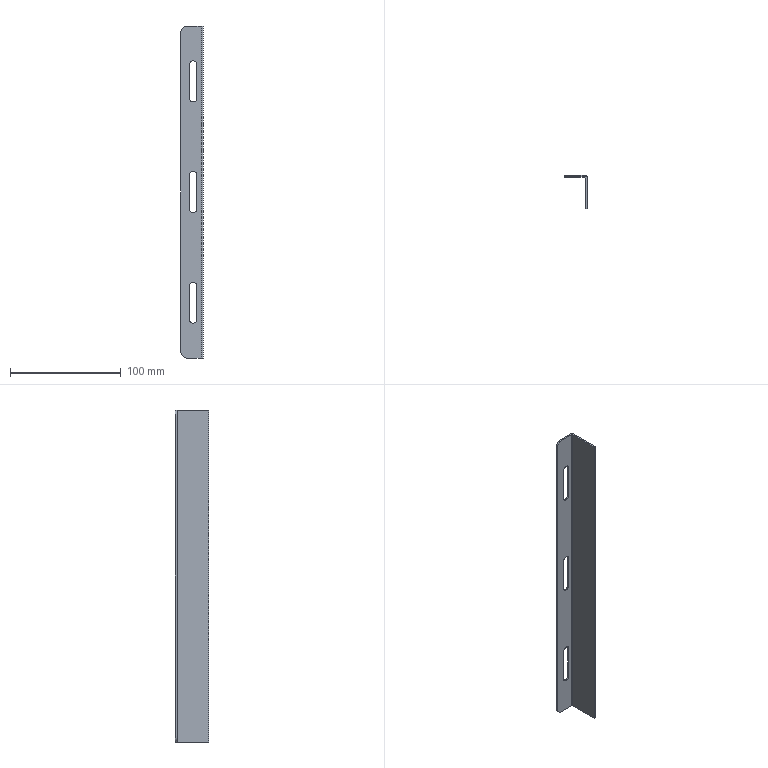Part | SolidWorks | features Cut 1, Fillet 1, FlatPattern 1, SMBaseFlange 1, SheetMetal 1 | 1 solid | 31 faces | box 20 x 30 x 300 mm | volume 20507 mm3 | plane 18 | cylinder 13 | commonest cylinder face diameters 7 x9 10 x2 0.4 x1 3.4 x1
STEP:
#1=CARTESIAN_POINT('',(-9.,-1.5,118.5));
#2=VERTEX_POINT('',#1);
#3=CARTESIAN_POINT('',(-5.5,-1.5,115.));
#4=VERTEX_POINT('',#3);
#5=CARTESIAN_POINT('',(-9.,-1.5,115.));
#6=DIRECTION('',(0.,1.,0.));
#7=DIRECTION('',(-1.,0.,0.));
#8=AXIS2_PLACEMENT_3D('',#5,#6,#7);
#9=CIRCLE('',#8,3.5);
#10=EDGE_CURVE('',#2,#4,#9,.T.);
#11=ORIENTED_EDGE('',*,*,#10,.F.);
#12=CARTESIAN_POINT('',(-9.,0.,118.5));
#13=VERTEX_POINT('',#12);
#14=CARTESIAN_POINT('',(-9.,-10.,118.5));
#15=DIRECTION('',(0.,1.,0.));
#16=VECTOR('',#15,1000.);
#17=LINE('',#14,#16);
#18=EDGE_CURVE('',#2,#13,#17,.T.);
#19=ORIENTED_EDGE('',*,*,#18,.T.);
#20=CARTESIAN_POINT('',(-5.5,0.,115.));
#21=VERTEX_POINT('',#20);
#22=CARTESIAN_POINT('',(-9.,0.,115.));
#23=DIRECTION('',(0.,1.,0.));
#24=DIRECTION('',(0.,0.,-1.));
#25=AXIS2_PLACEMENT_3D('',#22,#23,#24);
#26=CIRCLE('',#25,3.5);
#27=EDGE_CURVE('',#13,#21,#26,.T.);
#28=ORIENTED_EDGE('',*,*,#27,.T.);
#29=CARTESIAN_POINT('',(-5.5,-10.,115.));
#30=DIRECTION('',(0.,1.,0.));
#31=VECTOR('',#30,1000.);
#32=LINE('',#29,#31);
#33=EDGE_CURVE('',#4,#21,#32,.T.);
#34=ORIENTED_EDGE('',*,*,#33,.F.);
#35=EDGE_LOOP('',(#11,#19,#28,#34));
#36=FACE_OUTER_BOUND('',#35,.T.);
#37=CARTESIAN_POINT('',(-9.,-10.,115.));
#38=DIRECTION('',(0.,1.,0.));
#39=DIRECTION('',(0.,0.,1.));
#40=AXIS2_PLACEMENT_3D('',#37,#38,#39);
#41=CYLINDRICAL_SURFACE('',#40,3.5);
#42=ADVANCED_FACE('',(#36),#41,.F.);
#43=CARTESIAN_POINT('',(-9.,-1.5,-81.5));
#44=VERTEX_POINT('',#43);
#45=CARTESIAN_POINT('',(-5.5,-1.5,-85.));
#46=VERTEX_POINT('',#45);
#47=CARTESIAN_POINT('',(-9.,-1.5,-85.));
#48=DIRECTION('',(0.,1.,0.));
#49=DIRECTION('',(-1.,0.,0.));
#50=AXIS2_PLACEMENT_3D('',#47,#48,#49);
#51=CIRCLE('',#50,3.5);
#52=EDGE_CURVE('',#44,#46,#51,.T.);
#53=ORIENTED_EDGE('',*,*,#52,.F.);
#54=CARTESIAN_POINT('',(-9.,0.,-81.5));
#55=VERTEX_POINT('',#54);
#56=CARTESIAN_POINT('',(-9.,-10.,-81.5));
#57=DIRECTION('',(0.,1.,0.));
#58=VECTOR('',#57,1000.);
#59=LINE('',#56,#58);
#60=EDGE_CURVE('',#44,#55,#59,.T.);
#61=ORIENTED_EDGE('',*,*,#60,.T.);
#62=CARTESIAN_POINT('',(-5.5,0.,-85.));
#63=VERTEX_POINT('',#62);
#64=CARTESIAN_POINT('',(-9.,0.,-85.));
#65=DIRECTION('',(0.,1.,0.));
#66=DIRECTION('',(0.,0.,1.));
#67=AXIS2_PLACEMENT_3D('',#64,#65,#66);
#68=CIRCLE('',#67,3.5);
#69=EDGE_CURVE('',#55,#63,#68,.T.);
#70=ORIENTED_EDGE('',*,*,#69,.T.);
#71=CARTESIAN_POINT('',(-5.5,-10.,-85.));
#72=DIRECTION('',(0.,1.,0.));
#73=VECTOR('',#72,1000.);
#74=LINE('',#71,#73);
#75=EDGE_CURVE('',#46,#63,#74,.T.);
#76=ORIENTED_EDGE('',*,*,#75,.F.);
#77=EDGE_LOOP('',(#53,#61,#70,#76));
#78=FACE_OUTER_BOUND('',#77,.T.);
#79=CARTESIAN_POINT('',(-9.,-10.,-85.));
#80=DIRECTION('',(0.,1.,0.));
#81=DIRECTION('',(0.,0.,1.));
#82=AXIS2_PLACEMENT_3D('',#79,#80,#81);
#83=CYLINDRICAL_SURFACE('',#82,3.5);
#84=ADVANCED_FACE('',(#78),#83,.F.);
#85=CARTESIAN_POINT('',(-9.,-1.5,18.5));
#86=VERTEX_POINT('',#85);
#87=CARTESIAN_POINT('',(-5.5,-1.5,15.));
#88=VERTEX_POINT('',#87);
#89=CARTESIAN_POINT('',(-9.,-1.5,15.));
#90=DIRECTION('',(0.,1.,0.));
#91=DIRECTION('',(-1.,0.,0.));
#92=AXIS2_PLACEMENT_3D('',#89,#90,#91);
#93=CIRCLE('',#92,3.5);
#94=EDGE_CURVE('',#86,#88,#93,.T.);
#95=ORIENTED_EDGE('',*,*,#94,.F.);
#96=CARTESIAN_POINT('',(-9.,0.,18.5));
#97=VERTEX_POINT('',#96);
#98=CARTESIAN_POINT('',(-9.,-10.,18.5));
#99=DIRECTION('',(0.,1.,0.));
#100=VECTOR('',#99,1000.);
#101=LINE('',#98,#100);
#102=EDGE_CURVE('',#86,#97,#101,.T.);
#103=ORIENTED_EDGE('',*,*,#102,.T.);
#104=CARTESIAN_POINT('',(-5.5,0.,15.));
#105=VERTEX_POINT('',#104);
#106=CARTESIAN_POINT('',(-9.,0.,15.));
#107=DIRECTION('',(0.,1.,0.));
#108=DIRECTION('',(0.,0.,1.));
#109=AXIS2_PLACEMENT_3D('',#106,#107,#108);
#110=CIRCLE('',#109,3.5);
#111=EDGE_CURVE('',#97,#105,#110,.T.);
#112=ORIENTED_EDGE('',*,*,#111,.T.);
#113=CARTESIAN_POINT('',(-5.5,-10.,15.));
#114=DIRECTION('',(0.,1.,0.));
#115=VECTOR('',#114,1000.);
#116=LINE('',#113,#115);
#117=EDGE_CURVE('',#88,#105,#116,.T.);
#118=ORIENTED_EDGE('',*,*,#117,.F.);
#119=EDGE_LOOP('',(#95,#103,#112,#118));
#120=FACE_OUTER_BOUND('',#119,.T.);
#121=CARTESIAN_POINT('',(-9.,-10.,15.));
#122=DIRECTION('',(0.,1.,0.));
#123=DIRECTION('',(0.,0.,1.));
#124=AXIS2_PLACEMENT_3D('',#121,#122,#123);
#125=CYLINDRICAL_SURFACE('',#124,3.5);
#126=ADVANCED_FACE('',(#120),#125,.F.);
#127=CARTESIAN_POINT('',(0.,-1.7,150.));
#128=VERTEX_POINT('',#127);
#129=CARTESIAN_POINT('',(-1.5,-1.7,150.));
#130=VERTEX_POINT('',#129);
#131=CARTESIAN_POINT('',(0.,-1.7,150.));
#132=DIRECTION('',(-1.,0.,0.));
#133=VECTOR('',#132,1000.);
#134=LINE('',#131,#133);
#135=EDGE_CURVE('',#128,#130,#134,.T.);
#136=ORIENTED_EDGE('',*,*,#135,.F.);
#137=CARTESIAN_POINT('',(-1.7,0.,150.));
#138=VERTEX_POINT('',#137);
#139=CARTESIAN_POINT('',(-1.7,-1.7,150.));
#140=DIRECTION('',(0.,0.,-1.));
#141=DIRECTION('',(1.,0.,0.));
#142=AXIS2_PLACEMENT_3D('',#139,#140,#141);
#143=CIRCLE('',#142,1.7);
#144=EDGE_CURVE('',#138,#128,#143,.T.);
#145=ORIENTED_EDGE('',*,*,#144,.F.);
#146=CARTESIAN_POINT('',(-1.7,-1.5,150.));
#147=VERTEX_POINT('',#146);
#148=CARTESIAN_POINT('',(-1.7,-1.5,150.));
#149=DIRECTION('',(0.,1.,0.));
#150=VECTOR('',#149,1000.);
#151=LINE('',#148,#150);
#152=EDGE_CURVE('',#147,#138,#151,.T.);
#153=ORIENTED_EDGE('',*,*,#152,.F.);
#154=CARTESIAN_POINT('',(-1.7,-1.7,150.));
#155=DIRECTION('',(0.,0.,-1.));
#156=DIRECTION('',(1.,0.,0.));
#157=AXIS2_PLACEMENT_3D('',#154,#155,#156);
#158=CIRCLE('',#157,0.2);
#159=EDGE_CURVE('',#147,#130,#158,.T.);
#160=ORIENTED_EDGE('',*,*,#159,.T.);
#161=EDGE_LOOP('',(#136,#145,#153,#160));
#162=FACE_OUTER_BOUND('',#161,.T.);
#163=CARTESIAN_POINT('',(0.,-1.7,150.));
#164=DIRECTION('',(0.,0.,1.));
#165=DIRECTION('',(1.,0.,0.));
#166=AXIS2_PLACEMENT_3D('',#163,#164,#165);
#167=PLANE('',#166);
#168=ADVANCED_FACE('',(#162),#167,.T.);
#169=CARTESIAN_POINT('',(0.,-30.,150.));
#170=VERTEX_POINT('',#169);
#171=CARTESIAN_POINT('',(0.,0.,150.));
#172=DIRECTION('',(0.,-1.,0.));
#173=VECTOR('',#172,1000.);
#174=LINE('',#171,#173);
#175=EDGE_CURVE('',#128,#170,#174,.T.);
#176=ORIENTED_EDGE('',*,*,#175,.F.);
#177=ORIENTED_EDGE('',*,*,#135,.T.);
#178=CARTESIAN_POINT('',(-1.5,-30.,150.));
#179=VERTEX_POINT('',#178);
#180=CARTESIAN_POINT('',(-1.5,0.,150.));
#181=DIRECTION('',(0.,-1.,0.));
#182=VECTOR('',#181,1000.);
#183=LINE('',#180,#182);
#184=EDGE_CURVE('',#130,#179,#183,.T.);
#185=ORIENTED_EDGE('',*,*,#184,.T.);
#186=CARTESIAN_POINT('',(0.,-30.,150.));
#187=DIRECTION('',(-1.,0.,0.));
#188=VECTOR('',#187,1000.);
#189=LINE('',#186,#188);
#190=EDGE_CURVE('',#170,#179,#189,.T.);
#191=ORIENTED_EDGE('',*,*,#190,.F.);
#192=EDGE_LOOP('',(#176,#177,#185,#191));
#193=FACE_OUTER_BOUND('',#192,.T.);
#194=CARTESIAN_POINT('',(-1.7,-1.5,150.));
#195=DIRECTION('',(0.,0.,1.));
#196=DIRECTION('',(1.,0.,0.));
#197=AXIS2_PLACEMENT_3D('',#194,#195,#196);
#198=PLANE('',#197);
#199=ADVANCED_FACE('',(#193),#198,.T.);
#200=CARTESIAN_POINT('',(-1.7,0.,-150.));
#201=VERTEX_POINT('',#200);
#202=CARTESIAN_POINT('',(-1.7,-1.5,-150.));
#203=VERTEX_POINT('',#202);
#204=CARTESIAN_POINT('',(-1.7,0.,-150.));
#205=DIRECTION('',(0.,-1.,0.));
#206=VECTOR('',#205,1000.);
#207=LINE('',#204,#206);
#208=EDGE_CURVE('',#201,#203,#207,.T.);
#209=ORIENTED_EDGE('',*,*,#208,.F.);
#210=CARTESIAN_POINT('',(0.,-1.7,-150.));
#211=VERTEX_POINT('',#210);
#212=CARTESIAN_POINT('',(-1.7,-1.7,-150.));
#213=DIRECTION('',(0.,0.,-1.));
#214=DIRECTION('',(1.,0.,0.));
#215=AXIS2_PLACEMENT_3D('',#212,#213,#214);
#216=CIRCLE('',#215,1.7);
#217=EDGE_CURVE('',#201,#211,#216,.T.);
#218=ORIENTED_EDGE('',*,*,#217,.T.);
#219=CARTESIAN_POINT('',(-1.5,-1.7,-150.));
#220=VERTEX_POINT('',#219);
#221=CARTESIAN_POINT('',(-1.5,-1.7,-150.));
#222=DIRECTION('',(1.,0.,0.));
#223=VECTOR('',#222,1000.);
#224=LINE('',#221,#223);
#225=EDGE_CURVE('',#220,#211,#224,.T.);
#226=ORIENTED_EDGE('',*,*,#225,.F.);
#227=CARTESIAN_POINT('',(-1.7,-1.7,-150.));
#228=DIRECTION('',(0.,0.,-1.));
#229=DIRECTION('',(1.,0.,0.));
#230=AXIS2_PLACEMENT_3D('',#227,#228,#229);
#231=CIRCLE('',#230,0.2);
#232=EDGE_CURVE('',#203,#220,#231,.T.);
#233=ORIENTED_EDGE('',*,*,#232,.F.);
#234=EDGE_LOOP('',(#209,#218,#226,#233));
#235=FACE_OUTER_BOUND('',#234,.T.);
#236=CARTESIAN_POINT('',(-1.7,0.,-150.));
#237=DIRECTION('',(0.,0.,-1.));
#238=DIRECTION('',(-1.,0.,0.));
#239=AXIS2_PLACEMENT_3D('',#236,#237,#238);
#240=PLANE('',#239);
#241=ADVANCED_FACE('',(#235),#240,.T.);
#242=CARTESIAN_POINT('',(-15.,-1.5,-150.));
#243=VERTEX_POINT('',#242);
#244=CARTESIAN_POINT('',(0.,-1.5,-150.));
#245=DIRECTION('',(1.,0.,0.));
#246=VECTOR('',#245,1000.);
#247=LINE('',#244,#246);
#248=EDGE_CURVE('',#243,#203,#247,.T.);
#249=ORIENTED_EDGE('',*,*,#248,.F.);
#250=CARTESIAN_POINT('',(-15.,0.,-150.));
#251=VERTEX_POINT('',#250);
#252=CARTESIAN_POINT('',(-15.,-1.7,-150.));
#253=DIRECTION('',(0.,1.,0.));
#254=VECTOR('',#253,1000.);
#255=LINE('',#252,#254);
#256=EDGE_CURVE('',#243,#251,#255,.T.);
#257=ORIENTED_EDGE('',*,*,#256,.T.);
#258=CARTESIAN_POINT('',(0.,0.,-150.));
#259=DIRECTION('',(1.,0.,0.));
#260=VECTOR('',#259,1000.);
#261=LINE('',#258,#260);
#262=EDGE_CURVE('',#251,#201,#261,.T.);
#263=ORIENTED_EDGE('',*,*,#262,.T.);
#264=ORIENTED_EDGE('',*,*,#208,.T.);
#265=EDGE_LOOP('',(#249,#257,#263,#264));
#266=FACE_OUTER_BOUND('',#265,.T.);
#267=CARTESIAN_POINT('',(-1.5,-1.7,-150.));
#268=DIRECTION('',(0.,0.,-1.));
#269=DIRECTION('',(-1.,0.,0.));
#270=AXIS2_PLACEMENT_3D('',#267,#268,#269);
#271=PLANE('',#270);
#272=ADVANCED_FACE('',(#266),#271,.T.);
#273=CARTESIAN_POINT('',(-1.5,-30.,-150.));
#274=VERTEX_POINT('',#273);
#275=CARTESIAN_POINT('',(-1.5,0.,-150.));
#276=DIRECTION('',(0.,-1.,0.));
#277=VECTOR('',#276,1000.);
#278=LINE('',#275,#277);
#279=EDGE_CURVE('',#220,#274,#278,.T.);
#280=ORIENTED_EDGE('',*,*,#279,.T.);
#281=CARTESIAN_POINT('',(-1.5,-30.,150.));
#282=DIRECTION('',(0.,0.,-1.));
#283=VECTOR('',#282,1000.);
#284=LINE('',#281,#283);
#285=EDGE_CURVE('',#179,#274,#284,.T.);
#286=ORIENTED_EDGE('',*,*,#285,.F.);
#287=ORIENTED_EDGE('',*,*,#184,.F.);
#288=CARTESIAN_POINT('',(-1.5,-1.7,150.));
#289=DIRECTION('',(0.,0.,-1.));
#290=VECTOR('',#289,1000.);
#291=LINE('',#288,#290);
#292=EDGE_CURVE('',#130,#220,#291,.T.);
#293=ORIENTED_EDGE('',*,*,#292,.T.);
#294=EDGE_LOOP('',(#280,#286,#287,#293));
#295=FACE_OUTER_BOUND('',#294,.T.);
#296=CARTESIAN_POINT('',(-1.5,0.,150.));
#297=DIRECTION('',(1.,0.,0.));
#298=DIRECTION('',(0.,1.,0.));
#299=AXIS2_PLACEMENT_3D('',#296,#297,#298);
#300=PLANE('',#299);
#301=ADVANCED_FACE('',(#295),#300,.F.);
#302=CARTESIAN_POINT('',(0.,-30.,-150.));
#303=VERTEX_POINT('',#302);
#304=CARTESIAN_POINT('',(0.,-30.,-150.));
#305=DIRECTION('',(-1.,0.,0.));
#306=VECTOR('',#305,1000.);
#307=LINE('',#304,#306);
#308=EDGE_CURVE('',#303,#274,#307,.T.);
#309=ORIENTED_EDGE('',*,*,#308,.F.);
#310=CARTESIAN_POINT('',(0.,-30.,150.));
#311=DIRECTION('',(0.,0.,-1.));
#312=VECTOR('',#311,1000.);
#313=LINE('',#310,#312);
#314=EDGE_CURVE('',#170,#303,#313,.T.);
#315=ORIENTED_EDGE('',*,*,#314,.F.);
#316=ORIENTED_EDGE('',*,*,#190,.T.);
#317=ORIENTED_EDGE('',*,*,#285,.T.);
#318=EDGE_LOOP('',(#309,#315,#316,#317));
#319=FACE_OUTER_BOUND('',#318,.T.);
#320=CARTESIAN_POINT('',(0.,-30.,150.));
#321=DIRECTION('',(0.,-1.,0.));
#322=DIRECTION('',(0.,0.,-1.));
#323=AXIS2_PLACEMENT_3D('',#320,#321,#322);
#324=PLANE('',#323);
#325=ADVANCED_FACE('',(#319),#324,.T.);
#326=CARTESIAN_POINT('',(0.,0.,-150.));
#327=DIRECTION('',(0.,-1.,0.));
#328=VECTOR('',#327,1000.);
#329=LINE('',#326,#328);
#330=EDGE_CURVE('',#211,#303,#329,.T.);
#331=ORIENTED_EDGE('',*,*,#330,.F.);
#332=CARTESIAN_POINT('',(0.,-1.7,150.));
#333=DIRECTION('',(0.,0.,-1.));
#334=VECTOR('',#333,1000.);
#335=LINE('',#332,#334);
#336=EDGE_CURVE('',#128,#211,#335,.T.);
#337=ORIENTED_EDGE('',*,*,#336,.F.);
#338=ORIENTED_EDGE('',*,*,#175,.T.);
#339=ORIENTED_EDGE('',*,*,#314,.T.);
#340=EDGE_LOOP('',(#331,#337,#338,#339));
#341=FACE_OUTER_BOUND('',#340,.T.);
#342=CARTESIAN_POINT('',(0.,0.,150.));
#343=DIRECTION('',(1.,0.,0.));
#344=DIRECTION('',(0.,1.,0.));
#345=AXIS2_PLACEMENT_3D('',#342,#343,#344);
#346=PLANE('',#345);
#347=ADVANCED_FACE('',(#341),#346,.T.);
#348=ORIENTED_EDGE('',*,*,#217,.F.);
#349=CARTESIAN_POINT('',(-1.7,0.,150.));
#350=DIRECTION('',(0.,0.,-1.));
#351=VECTOR('',#350,1000.);
#352=LINE('',#349,#351);
#353=EDGE_CURVE('',#138,#201,#352,.T.);
#354=ORIENTED_EDGE('',*,*,#353,.F.);
#355=ORIENTED_EDGE('',*,*,#144,.T.);
#356=ORIENTED_EDGE('',*,*,#336,.T.);
#357=EDGE_LOOP('',(#348,#354,#355,#356));
#358=FACE_OUTER_BOUND('',#357,.T.);
#359=CARTESIAN_POINT('',(-1.7,-1.7,150.));
#360=DIRECTION('',(0.,0.,-1.));
#361=DIRECTION('',(-1.,0.,0.));
#362=AXIS2_PLACEMENT_3D('',#359,#360,#361);
#363=CYLINDRICAL_SURFACE('',#362,1.7);
#364=ADVANCED_FACE('',(#358),#363,.T.);
#365=CARTESIAN_POINT('',(-5.5,0.,85.));
#366=VERTEX_POINT('',#365);
#367=CARTESIAN_POINT('',(-12.5,0.,85.));
#368=VERTEX_POINT('',#367);
#369=CARTESIAN_POINT('',(-9.,0.,85.));
#370=DIRECTION('',(0.,1.,0.));
#371=DIRECTION('',(0.,0.,-1.));
#372=AXIS2_PLACEMENT_3D('',#369,#370,#371);
#373=CIRCLE('',#372,3.5);
#374=EDGE_CURVE('',#366,#368,#373,.T.);
#375=ORIENTED_EDGE('',*,*,#374,.F.);
#376=CARTESIAN_POINT('',(-5.5,0.,85.));
#377=DIRECTION('',(0.,0.,-1.));
#378=VECTOR('',#377,1000.);
#379=LINE('',#376,#378);
#380=EDGE_CURVE('',#21,#366,#379,.T.);
#381=ORIENTED_EDGE('',*,*,#380,.F.);
#382=ORIENTED_EDGE('',*,*,#27,.F.);
#383=CARTESIAN_POINT('',(-12.5,0.,115.));
#384=VERTEX_POINT('',#383);
#385=CARTESIAN_POINT('',(-9.,0.,115.));
#386=DIRECTION('',(0.,1.,0.));
#387=DIRECTION('',(0.,0.,-1.));
#388=AXIS2_PLACEMENT_3D('',#385,#386,#387);
#389=CIRCLE('',#388,3.5);
#390=EDGE_CURVE('',#384,#13,#389,.T.);
#391=ORIENTED_EDGE('',*,*,#390,.F.);
#392=CARTESIAN_POINT('',(-12.5,0.,85.));
#393=DIRECTION('',(0.,0.,1.));
#394=VECTOR('',#393,1000.);
#395=LINE('',#392,#394);
#396=EDGE_CURVE('',#368,#384,#395,.T.);
#397=ORIENTED_EDGE('',*,*,#396,.F.);
#398=EDGE_LOOP('',(#375,#381,#382,#391,#397));
#399=FACE_BOUND('',#398,.T.);
#400=CARTESIAN_POINT('',(-12.5,0.,-85.));
#401=VERTEX_POINT('',#400);
#402=CARTESIAN_POINT('',(-9.,0.,-85.));
#403=DIRECTION('',(0.,1.,0.));
#404=DIRECTION('',(0.,0.,1.));
#405=AXIS2_PLACEMENT_3D('',#402,#403,#404);
#406=CIRCLE('',#405,3.5);
#407=EDGE_CURVE('',#401,#55,#406,.T.);
#408=ORIENTED_EDGE('',*,*,#407,.F.);
#409=CARTESIAN_POINT('',(-12.5,0.,-115.));
#410=VERTEX_POINT('',#409);
#411=CARTESIAN_POINT('',(-12.5,0.,-85.));
#412=DIRECTION('',(0.,0.,1.));
#413=VECTOR('',#412,1000.);
#414=LINE('',#411,#413);
#415=EDGE_CURVE('',#410,#401,#414,.T.);
#416=ORIENTED_EDGE('',*,*,#415,.F.);
#417=CARTESIAN_POINT('',(-5.5,0.,-115.));
#418=VERTEX_POINT('',#417);
#419=CARTESIAN_POINT('',(-9.,0.,-115.));
#420=DIRECTION('',(0.,1.,0.));
#421=DIRECTION('',(0.,0.,1.));
#422=AXIS2_PLACEMENT_3D('',#419,#420,#421);
#423=CIRCLE('',#422,3.5);
#424=EDGE_CURVE('',#418,#410,#423,.T.);
#425=ORIENTED_EDGE('',*,*,#424,.F.);
#426=CARTESIAN_POINT('',(-5.5,0.,-85.));
#427=DIRECTION('',(0.,0.,-1.));
#428=VECTOR('',#427,1000.);
#429=LINE('',#426,#428);
#430=EDGE_CURVE('',#63,#418,#429,.T.);
#431=ORIENTED_EDGE('',*,*,#430,.F.);
#432=ORIENTED_EDGE('',*,*,#69,.F.);
#433=EDGE_LOOP('',(#408,#416,#425,#431,#432));
#434=FACE_BOUND('',#433,.T.);
#435=CARTESIAN_POINT('',(-12.5,0.,15.));
#436=VERTEX_POINT('',#435);
#437=CARTESIAN_POINT('',(-9.,0.,15.));
#438=DIRECTION('',(0.,1.,0.));
#439=DIRECTION('',(0.,0.,1.));
#440=AXIS2_PLACEMENT_3D('',#437,#438,#439);
#441=CIRCLE('',#440,3.5);
#442=EDGE_CURVE('',#436,#97,#441,.T.);
#443=ORIENTED_EDGE('',*,*,#442,.F.);
#444=CARTESIAN_POINT('',(-12.5,0.,-15.));
#445=VERTEX_POINT('',#444);
#446=CARTESIAN_POINT('',(-12.5,0.,15.));
#447=DIRECTION('',(0.,0.,1.));
#448=VECTOR('',#447,1000.);
#449=LINE('',#446,#448);
#450=EDGE_CURVE('',#445,#436,#449,.T.);
#451=ORIENTED_EDGE('',*,*,#450,.F.);
#452=CARTESIAN_POINT('',(-5.5,0.,-15.));
#453=VERTEX_POINT('',#452);
#454=CARTESIAN_POINT('',(-9.,0.,-15.));
#455=DIRECTION('',(0.,1.,0.));
#456=DIRECTION('',(0.,0.,1.));
#457=AXIS2_PLACEMENT_3D('',#454,#455,#456);
#458=CIRCLE('',#457,3.5);
#459=EDGE_CURVE('',#453,#445,#458,.T.);
#460=ORIENTED_EDGE('',*,*,#459,.F.);
#461=CARTESIAN_POINT('',(-5.5,0.,15.));
#462=DIRECTION('',(0.,0.,-1.));
#463=VECTOR('',#462,1000.);
#464=LINE('',#461,#463);
#465=EDGE_CURVE('',#105,#453,#464,.T.);
#466=ORIENTED_EDGE('',*,*,#465,.F.);
#467=ORIENTED_EDGE('',*,*,#111,.F.);
#468=EDGE_LOOP('',(#443,#451,#460,#466,#467));
#469=FACE_BOUND('',#468,.T.);
#470=ORIENTED_EDGE('',*,*,#262,.F.);
#471=CARTESIAN_POINT('',(-20.,0.,-145.));
#472=VERTEX_POINT('',#471);
#473=CARTESIAN_POINT('',(-15.,0.,-145.));
#474=DIRECTION('',(0.,1.,0.));
#475=DIRECTION('',(-1.,0.,0.));
#476=AXIS2_PLACEMENT_3D('',#473,#474,#475);
#477=CIRCLE('',#476,5.);
#478=EDGE_CURVE('',#251,#472,#477,.T.);
#479=ORIENTED_EDGE('',*,*,#478,.T.);
#480=CARTESIAN_POINT('',(-20.,0.,145.));
#481=VERTEX_POINT('',#480);
#482=CARTESIAN_POINT('',(-20.,0.,150.));
#483=DIRECTION('',(0.,0.,-1.));
#484=VECTOR('',#483,1000.);
#485=LINE('',#482,#484);
#486=EDGE_CURVE('',#481,#472,#485,.T.);
#487=ORIENTED_EDGE('',*,*,#486,.F.);
#488=CARTESIAN_POINT('',(-15.,0.,150.));
#489=VERTEX_POINT('',#488);
#490=CARTESIAN_POINT('',(-15.,0.,145.));
#491=DIRECTION('',(0.,1.,0.));
#492=DIRECTION('',(-1.,0.,0.));
#493=AXIS2_PLACEMENT_3D('',#490,#491,#492);
#494=CIRCLE('',#493,5.);
#495=EDGE_CURVE('',#481,#489,#494,.T.);
#496=ORIENTED_EDGE('',*,*,#495,.T.);
#497=CARTESIAN_POINT('',(0.,0.,150.));
#498=DIRECTION('',(1.,0.,0.));
#499=VECTOR('',#498,1000.);
#500=LINE('',#497,#499);
#501=EDGE_CURVE('',#489,#138,#500,.T.);
#502=ORIENTED_EDGE('',*,*,#501,.T.);
#503=ORIENTED_EDGE('',*,*,#353,.T.);
#504=EDGE_LOOP('',(#470,#479,#487,#496,#502,#503));
#505=FACE_OUTER_BOUND('',#504,.T.);
#506=CARTESIAN_POINT('',(0.,0.,150.));
#507=DIRECTION('',(0.,1.,0.));
#508=DIRECTION('',(-1.,0.,0.));
#509=AXIS2_PLACEMENT_3D('',#506,#507,#508);
#510=PLANE('',#509);
#511=ADVANCED_FACE('',(#399,#434,#469,#505),#510,.T.);
#512=ORIENTED_EDGE('',*,*,#486,.T.);
#513=CARTESIAN_POINT('',(-20.,-1.5,-145.));
#514=VERTEX_POINT('',#513);
#515=CARTESIAN_POINT('',(-20.,-1.5,-145.));
#516=DIRECTION('',(0.,-1.,0.));
#517=VECTOR('',#516,1000.);
#518=LINE('',#515,#517);
#519=EDGE_CURVE('',#472,#514,#518,.T.);
#520=ORIENTED_EDGE('',*,*,#519,.T.);
#521=CARTESIAN_POINT('',(-20.,-1.5,145.));
#522=VERTEX_POINT('',#521);
#523=CARTESIAN_POINT('',(-20.,-1.5,150.));
#524=DIRECTION('',(0.,0.,-1.));
#525=VECTOR('',#524,1000.);
#526=LINE('',#523,#525);
#527=EDGE_CURVE('',#522,#514,#526,.T.);
#528=ORIENTED_EDGE('',*,*,#527,.F.);
#529=CARTESIAN_POINT('',(-20.,-1.5,145.));
#530=DIRECTION('',(0.,1.,0.));
#531=VECTOR('',#530,1000.);
#532=LINE('',#529,#531);
#533=EDGE_CURVE('',#522,#481,#532,.T.);
#534=ORIENTED_EDGE('',*,*,#533,.T.);
#535=EDGE_LOOP('',(#512,#520,#528,#534));
#536=FACE_OUTER_BOUND('',#535,.T.);
#537=CARTESIAN_POINT('',(-20.,-1.5,150.));
#538=DIRECTION('',(-1.,0.,0.));
#539=DIRECTION('',(0.,0.,1.));
#540=AXIS2_PLACEMENT_3D('',#537,#538,#539);
#541=PLANE('',#540);
#542=ADVANCED_FACE('',(#536),#541,.T.);
#543=CARTESIAN_POINT('',(-5.5,-1.5,85.));
#544=VERTEX_POINT('',#543);
#545=CARTESIAN_POINT('',(-5.5,-1.5,150.));
#546=DIRECTION('',(0.,0.,-1.));
#547=VECTOR('',#546,1000.);
#548=LINE('',#545,#547);
#549=EDGE_CURVE('',#4,#544,#548,.T.);
#550=ORIENTED_EDGE('',*,*,#549,.T.);
#551=CARTESIAN_POINT('',(-12.5,-1.5,85.));
#552=VERTEX_POINT('',#551);
#553=CARTESIAN_POINT('',(-9.,-1.5,85.));
#554=DIRECTION('',(0.,1.,0.));
#555=DIRECTION('',(-1.,0.,0.));
#556=AXIS2_PLACEMENT_3D('',#553,#554,#555);
#557=CIRCLE('',#556,3.5);
#558=EDGE_CURVE('',#544,#552,#557,.T.);
#559=ORIENTED_EDGE('',*,*,#558,.T.);
#560=CARTESIAN_POINT('',(-12.5,-1.5,115.));
#561=VERTEX_POINT('',#560);
#562=CARTESIAN_POINT('',(-12.5,-1.5,150.));
#563=DIRECTION('',(0.,0.,1.));
#564=VECTOR('',#563,1000.);
#565=LINE('',#562,#564);
#566=EDGE_CURVE('',#552,#561,#565,.T.);
#567=ORIENTED_EDGE('',*,*,#566,.T.);
#568=CARTESIAN_POINT('',(-9.,-1.5,115.));
#569=DIRECTION('',(0.,1.,0.));
#570=DIRECTION('',(-1.,0.,0.));
#571=AXIS2_PLACEMENT_3D('',#568,#569,#570);
#572=CIRCLE('',#571,3.5);
#573=EDGE_CURVE('',#561,#2,#572,.T.);
#574=ORIENTED_EDGE('',*,*,#573,.T.);
#575=ORIENTED_EDGE('',*,*,#10,.T.);
#576=EDGE_LOOP('',(#550,#559,#567,#574,#575));
#577=FACE_BOUND('',#576,.T.);
#578=CARTESIAN_POINT('',(-12.5,-1.5,-115.));
#579=VERTEX_POINT('',#578);
#580=CARTESIAN_POINT('',(-12.5,-1.5,-85.));
#581=VERTEX_POINT('',#580);
#582=CARTESIAN_POINT('',(-12.5,-1.5,150.));
#583=DIRECTION('',(0.,0.,1.));
#584=VECTOR('',#583,1000.);
#585=LINE('',#582,#584);
#586=EDGE_CURVE('',#579,#581,#585,.T.);
#587=ORIENTED_EDGE('',*,*,#586,.T.);
#588=CARTESIAN_POINT('',(-9.,-1.5,-85.));
#589=DIRECTION('',(0.,1.,0.));
#590=DIRECTION('',(-1.,0.,0.));
#591=AXIS2_PLACEMENT_3D('',#588,#589,#590);
#592=CIRCLE('',#591,3.5);
#593=EDGE_CURVE('',#581,#44,#592,.T.);
#594=ORIENTED_EDGE('',*,*,#593,.T.);
#595=ORIENTED_EDGE('',*,*,#52,.T.);
#596=CARTESIAN_POINT('',(-5.5,-1.5,-115.));
#597=VERTEX_POINT('',#596);
#598=CARTESIAN_POINT('',(-5.5,-1.5,150.));
#599=DIRECTION('',(0.,0.,-1.));
#600=VECTOR('',#599,1000.);
#601=LINE('',#598,#600);
#602=EDGE_CURVE('',#46,#597,#601,.T.);
#603=ORIENTED_EDGE('',*,*,#602,.T.);
#604=CARTESIAN_POINT('',(-9.,-1.5,-115.));
#605=DIRECTION('',(0.,1.,0.));
#606=DIRECTION('',(-1.,0.,0.));
#607=AXIS2_PLACEMENT_3D('',#604,#605,#606);
#608=CIRCLE('',#607,3.5);
#609=EDGE_CURVE('',#597,#579,#608,.T.);
#610=ORIENTED_EDGE('',*,*,#609,.T.);
#611=EDGE_LOOP('',(#587,#594,#595,#603,#610));
#612=FACE_BOUND('',#611,.T.);
#613=CARTESIAN_POINT('',(-12.5,-1.5,-15.));
#614=VERTEX_POINT('',#613);
#615=CARTESIAN_POINT('',(-12.5,-1.5,15.));
#616=VERTEX_POINT('',#615);
#617=CARTESIAN_POINT('',(-12.5,-1.5,150.));
#618=DIRECTION('',(0.,0.,1.));
#619=VECTOR('',#618,1000.);
#620=LINE('',#617,#619);
#621=EDGE_CURVE('',#614,#616,#620,.T.);
#622=ORIENTED_EDGE('',*,*,#621,.T.);
#623=CARTESIAN_POINT('',(-9.,-1.5,15.));
#624=DIRECTION('',(0.,1.,0.));
#625=DIRECTION('',(-1.,0.,0.));
#626=AXIS2_PLACEMENT_3D('',#623,#624,#625);
#627=CIRCLE('',#626,3.5);
#628=EDGE_CURVE('',#616,#86,#627,.T.);
#629=ORIENTED_EDGE('',*,*,#628,.T.);
#630=ORIENTED_EDGE('',*,*,#94,.T.);
#631=CARTESIAN_POINT('',(-5.5,-1.5,-15.));
#632=VERTEX_POINT('',#631);
#633=CARTESIAN_POINT('',(-5.5,-1.5,150.));
#634=DIRECTION('',(0.,0.,-1.));
#635=VECTOR('',#634,1000.);
#636=LINE('',#633,#635);
#637=EDGE_CURVE('',#88,#632,#636,.T.);
#638=ORIENTED_EDGE('',*,*,#637,.T.);
#639=CARTESIAN_POINT('',(-9.,-1.5,-15.));
#640=DIRECTION('',(0.,1.,0.));
#641=DIRECTION('',(-1.,0.,0.));
#642=AXIS2_PLACEMENT_3D('',#639,#640,#641);
#643=CIRCLE('',#642,3.5);
#644=EDGE_CURVE('',#632,#614,#643,.T.);
#645=ORIENTED_EDGE('',*,*,#644,.T.);
#646=EDGE_LOOP('',(#622,#629,#630,#638,#645));
#647=FACE_BOUND('',#646,.T.);
#648=ORIENTED_EDGE('',*,*,#527,.T.);
#649=CARTESIAN_POINT('',(-15.,-1.5,-145.));
#650=DIRECTION('',(0.,-1.,0.));
#651=DIRECTION('',(-1.,0.,0.));
#652=AXIS2_PLACEMENT_3D('',#649,#650,#651);
#653=CIRCLE('',#652,5.);
#654=EDGE_CURVE('',#514,#243,#653,.T.);
#655=ORIENTED_EDGE('',*,*,#654,.T.);
#656=ORIENTED_EDGE('',*,*,#248,.T.);
#657=CARTESIAN_POINT('',(-1.7,-1.5,150.));
#658=DIRECTION('',(0.,0.,-1.));
#659=VECTOR('',#658,1000.);
#660=LINE('',#657,#659);
#661=EDGE_CURVE('',#147,#203,#660,.T.);
#662=ORIENTED_EDGE('',*,*,#661,.F.);
#663=CARTESIAN_POINT('',(-15.,-1.5,150.));
#664=VERTEX_POINT('',#663);
#665=CARTESIAN_POINT('',(0.,-1.5,150.));
#666=DIRECTION('',(1.,0.,0.));
#667=VECTOR('',#666,1000.);
#668=LINE('',#665,#667);
#669=EDGE_CURVE('',#664,#147,#668,.T.);
#670=ORIENTED_EDGE('',*,*,#669,.F.);
#671=CARTESIAN_POINT('',(-15.,-1.5,145.));
#672=DIRECTION('',(0.,-1.,0.));
#673=DIRECTION('',(-1.,0.,0.));
#674=AXIS2_PLACEMENT_3D('',#671,#672,#673);
#675=CIRCLE('',#674,5.);
#676=EDGE_CURVE('',#664,#522,#675,.T.);
#677=ORIENTED_EDGE('',*,*,#676,.T.);
#678=EDGE_LOOP('',(#648,#655,#656,#662,#670,#677));
#679=FACE_OUTER_BOUND('',#678,.T.);
#680=CARTESIAN_POINT('',(0.,-1.5,150.));
#681=DIRECTION('',(0.,1.,0.));
#682=DIRECTION('',(-1.,0.,0.));
#683=AXIS2_PLACEMENT_3D('',#680,#681,#682);
#684=PLANE('',#683);
#685=ADVANCED_FACE('',(#577,#612,#647,#679),#684,.F.);
#686=ORIENTED_EDGE('',*,*,#232,.T.);
#687=ORIENTED_EDGE('',*,*,#292,.F.);
#688=ORIENTED_EDGE('',*,*,#159,.F.);
#689=ORIENTED_EDGE('',*,*,#661,.T.);
#690=EDGE_LOOP('',(#686,#687,#688,#689));
#691=FACE_OUTER_BOUND('',#690,.T.);
#692=CARTESIAN_POINT('',(-1.7,-1.7,150.));
#693=DIRECTION('',(0.,0.,-1.));
#694=DIRECTION('',(-1.,0.,0.));
#695=AXIS2_PLACEMENT_3D('',#692,#693,#694);
#696=CYLINDRICAL_SURFACE('',#695,0.2);
#697=ADVANCED_FACE('',(#691),#696,.F.);
#698=ORIENTED_EDGE('',*,*,#501,.F.);
#699=CARTESIAN_POINT('',(-15.,-1.7,150.));
#700=DIRECTION('',(0.,-1.,0.));
#701=VECTOR('',#700,1000.);
#702=LINE('',#699,#701);
#703=EDGE_CURVE('',#489,#664,#702,.T.);
#704=ORIENTED_EDGE('',*,*,#703,.T.);
#705=ORIENTED_EDGE('',*,*,#669,.T.);
#706=ORIENTED_EDGE('',*,*,#152,.T.);
#707=EDGE_LOOP('',(#698,#704,#705,#706));
#708=FACE_OUTER_BOUND('',#707,.T.);
#709=CARTESIAN_POINT('',(-1.7,-1.7,150.));
#710=DIRECTION('',(0.,0.,1.));
#711=DIRECTION('',(1.,0.,0.));
#712=AXIS2_PLACEMENT_3D('',#709,#710,#711);
#713=PLANE('',#712);
#714=ADVANCED_FACE('',(#708),#713,.T.);
#715=ORIENTED_EDGE('',*,*,#279,.F.);
#716=ORIENTED_EDGE('',*,*,#225,.T.);
#717=ORIENTED_EDGE('',*,*,#330,.T.);
#718=ORIENTED_EDGE('',*,*,#308,.T.);
#719=EDGE_LOOP('',(#715,#716,#717,#718));
#720=FACE_OUTER_BOUND('',#719,.T.);
#721=CARTESIAN_POINT('',(-1.7,-1.7,-150.));
#722=DIRECTION('',(0.,0.,1.));
#723=DIRECTION('',(1.,0.,0.));
#724=AXIS2_PLACEMENT_3D('',#721,#722,#723);
#725=PLANE('',#724);
#726=ADVANCED_FACE('',(#720),#725,.F.);
#727=ORIENTED_EDGE('',*,*,#102,.F.);
#728=ORIENTED_EDGE('',*,*,#628,.F.);
#729=CARTESIAN_POINT('',(-12.5,-10.,15.));
#730=DIRECTION('',(0.,1.,0.));
#731=VECTOR('',#730,1000.);
#732=LINE('',#729,#731);
#733=EDGE_CURVE('',#616,#436,#732,.T.);
#734=ORIENTED_EDGE('',*,*,#733,.T.);
#735=ORIENTED_EDGE('',*,*,#442,.T.);
#736=EDGE_LOOP('',(#727,#728,#734,#735));
#737=FACE_OUTER_BOUND('',#736,.T.);
#738=CARTESIAN_POINT('',(-9.,-10.,15.));
#739=DIRECTION('',(0.,1.,0.));
#740=DIRECTION('',(0.,0.,1.));
#741=AXIS2_PLACEMENT_3D('',#738,#739,#740);
#742=CYLINDRICAL_SURFACE('',#741,3.5);
#743=ADVANCED_FACE('',(#737),#742,.F.);
#744=CARTESIAN_POINT('',(-12.5,-10.,-15.));
#745=DIRECTION('',(0.,1.,0.));
#746=VECTOR('',#745,1000.);
#747=LINE('',#744,#746);
#748=EDGE_CURVE('',#614,#445,#747,.T.);
#749=ORIENTED_EDGE('',*,*,#748,.T.);
#750=ORIENTED_EDGE('',*,*,#450,.T.);
#751=ORIENTED_EDGE('',*,*,#733,.F.);
#752=ORIENTED_EDGE('',*,*,#621,.F.);
#753=EDGE_LOOP('',(#749,#750,#751,#752));
#754=FACE_OUTER_BOUND('',#753,.T.);
#755=CARTESIAN_POINT('',(-12.5,-10.,15.));
#756=DIRECTION('',(-1.,0.,0.));
#757=DIRECTION('',(0.,0.,1.));
#758=AXIS2_PLACEMENT_3D('',#755,#756,#757);
#759=PLANE('',#758);
#760=ADVANCED_FACE('',(#754),#759,.F.);
#761=CARTESIAN_POINT('',(-5.5,-10.,-15.));
#762=DIRECTION('',(0.,1.,0.));
#763=VECTOR('',#762,1000.);
#764=LINE('',#761,#763);
#765=EDGE_CURVE('',#632,#453,#764,.T.);
#766=ORIENTED_EDGE('',*,*,#765,.T.);
#767=ORIENTED_EDGE('',*,*,#459,.T.);
#768=ORIENTED_EDGE('',*,*,#748,.F.);
#769=ORIENTED_EDGE('',*,*,#644,.F.);
#770=EDGE_LOOP('',(#766,#767,#768,#769));
#771=FACE_OUTER_BOUND('',#770,.T.);
#772=CARTESIAN_POINT('',(-9.,-10.,-15.));
#773=DIRECTION('',(0.,1.,0.));
#774=DIRECTION('',(0.,0.,1.));
#775=AXIS2_PLACEMENT_3D('',#772,#773,#774);
#776=CYLINDRICAL_SURFACE('',#775,3.5);
#777=ADVANCED_FACE('',(#771),#776,.F.);
#778=ORIENTED_EDGE('',*,*,#117,.T.);
#779=ORIENTED_EDGE('',*,*,#465,.T.);
#780=ORIENTED_EDGE('',*,*,#765,.F.);
#781=ORIENTED_EDGE('',*,*,#637,.F.);
#782=EDGE_LOOP('',(#778,#779,#780,#781));
#783=FACE_OUTER_BOUND('',#782,.T.);
#784=CARTESIAN_POINT('',(-5.5,-10.,15.));
#785=DIRECTION('',(1.,0.,0.));
#786=DIRECTION('',(0.,0.,-1.));
#787=AXIS2_PLACEMENT_3D('',#784,#785,#786);
#788=PLANE('',#787);
#789=ADVANCED_FACE('',(#783),#788,.F.);
#790=ORIENTED_EDGE('',*,*,#60,.F.);
#791=ORIENTED_EDGE('',*,*,#593,.F.);
#792=CARTESIAN_POINT('',(-12.5,-10.,-85.));
#793=DIRECTION('',(0.,1.,0.));
#794=VECTOR('',#793,1000.);
#795=LINE('',#792,#794);
#796=EDGE_CURVE('',#581,#401,#795,.T.);
#797=ORIENTED_EDGE('',*,*,#796,.T.);
#798=ORIENTED_EDGE('',*,*,#407,.T.);
#799=EDGE_LOOP('',(#790,#791,#797,#798));
#800=FACE_OUTER_BOUND('',#799,.T.);
#801=CARTESIAN_POINT('',(-9.,-10.,-85.));
#802=DIRECTION('',(0.,1.,0.));
#803=DIRECTION('',(0.,0.,1.));
#804=AXIS2_PLACEMENT_3D('',#801,#802,#803);
#805=CYLINDRICAL_SURFACE('',#804,3.5);
#806=ADVANCED_FACE('',(#800),#805,.F.);
#807=CARTESIAN_POINT('',(-12.5,-10.,-115.));
#808=DIRECTION('',(0.,1.,0.));
#809=VECTOR('',#808,1000.);
#810=LINE('',#807,#809);
#811=EDGE_CURVE('',#579,#410,#810,.T.);
#812=ORIENTED_EDGE('',*,*,#811,.T.);
#813=ORIENTED_EDGE('',*,*,#415,.T.);
#814=ORIENTED_EDGE('',*,*,#796,.F.);
#815=ORIENTED_EDGE('',*,*,#586,.F.);
#816=EDGE_LOOP('',(#812,#813,#814,#815));
#817=FACE_OUTER_BOUND('',#816,.T.);
#818=CARTESIAN_POINT('',(-12.5,-10.,-85.));
#819=DIRECTION('',(-1.,0.,0.));
#820=DIRECTION('',(0.,0.,1.));
#821=AXIS2_PLACEMENT_3D('',#818,#819,#820);
#822=PLANE('',#821);
#823=ADVANCED_FACE('',(#817),#822,.F.);
#824=CARTESIAN_POINT('',(-5.5,-10.,-115.));
#825=DIRECTION('',(0.,1.,0.));
#826=VECTOR('',#825,1000.);
#827=LINE('',#824,#826);
#828=EDGE_CURVE('',#597,#418,#827,.T.);
#829=ORIENTED_EDGE('',*,*,#828,.T.);
#830=ORIENTED_EDGE('',*,*,#424,.T.);
#831=ORIENTED_EDGE('',*,*,#811,.F.);
#832=ORIENTED_EDGE('',*,*,#609,.F.);
#833=EDGE_LOOP('',(#829,#830,#831,#832));
#834=FACE_OUTER_BOUND('',#833,.T.);
#835=CARTESIAN_POINT('',(-9.,-10.,-115.));
#836=DIRECTION('',(0.,1.,0.));
#837=DIRECTION('',(0.,0.,1.));
#838=AXIS2_PLACEMENT_3D('',#835,#836,#837);
#839=CYLINDRICAL_SURFACE('',#838,3.5);
#840=ADVANCED_FACE('',(#834),#839,.F.);
#841=ORIENTED_EDGE('',*,*,#75,.T.);
#842=ORIENTED_EDGE('',*,*,#430,.T.);
#843=ORIENTED_EDGE('',*,*,#828,.F.);
#844=ORIENTED_EDGE('',*,*,#602,.F.);
#845=EDGE_LOOP('',(#841,#842,#843,#844));
#846=FACE_OUTER_BOUND('',#845,.T.);
#847=CARTESIAN_POINT('',(-5.5,-10.,-85.));
#848=DIRECTION('',(1.,0.,0.));
#849=DIRECTION('',(0.,0.,-1.));
#850=AXIS2_PLACEMENT_3D('',#847,#848,#849);
#851=PLANE('',#850);
#852=ADVANCED_FACE('',(#846),#851,.F.);
#853=CARTESIAN_POINT('',(-5.5,-10.,85.));
#854=DIRECTION('',(0.,1.,0.));
#855=VECTOR('',#854,1000.);
#856=LINE('',#853,#855);
#857=EDGE_CURVE('',#544,#366,#856,.T.);
#858=ORIENTED_EDGE('',*,*,#857,.T.);
#859=ORIENTED_EDGE('',*,*,#374,.T.);
#860=CARTESIAN_POINT('',(-12.5,-10.,85.));
#861=DIRECTION('',(0.,1.,0.));
#862=VECTOR('',#861,1000.);
#863=LINE('',#860,#862);
#864=EDGE_CURVE('',#552,#368,#863,.T.);
#865=ORIENTED_EDGE('',*,*,#864,.F.);
#866=ORIENTED_EDGE('',*,*,#558,.F.);
#867=EDGE_LOOP('',(#858,#859,#865,#866));
#868=FACE_OUTER_BOUND('',#867,.T.);
#869=CARTESIAN_POINT('',(-9.,-10.,85.));
#870=DIRECTION('',(0.,1.,0.));
#871=DIRECTION('',(0.,0.,1.));
#872=AXIS2_PLACEMENT_3D('',#869,#870,#871);
#873=CYLINDRICAL_SURFACE('',#872,3.5);
#874=ADVANCED_FACE('',(#868),#873,.F.);
#875=ORIENTED_EDGE('',*,*,#33,.T.);
#876=ORIENTED_EDGE('',*,*,#380,.T.);
#877=ORIENTED_EDGE('',*,*,#857,.F.);
#878=ORIENTED_EDGE('',*,*,#549,.F.);
#879=EDGE_LOOP('',(#875,#876,#877,#878));
#880=FACE_OUTER_BOUND('',#879,.T.);
#881=CARTESIAN_POINT('',(-5.5,-10.,85.));
#882=DIRECTION('',(1.,0.,0.));
#883=DIRECTION('',(0.,0.,-1.));
#884=AXIS2_PLACEMENT_3D('',#881,#882,#883);
#885=PLANE('',#884);
#886=ADVANCED_FACE('',(#880),#885,.F.);
#887=ORIENTED_EDGE('',*,*,#18,.F.);
#888=ORIENTED_EDGE('',*,*,#573,.F.);
#889=CARTESIAN_POINT('',(-12.5,-10.,115.));
#890=DIRECTION('',(0.,1.,0.));
#891=VECTOR('',#890,1000.);
#892=LINE('',#889,#891);
#893=EDGE_CURVE('',#561,#384,#892,.T.);
#894=ORIENTED_EDGE('',*,*,#893,.T.);
#895=ORIENTED_EDGE('',*,*,#390,.T.);
#896=EDGE_LOOP('',(#887,#888,#894,#895));
#897=FACE_OUTER_BOUND('',#896,.T.);
#898=CARTESIAN_POINT('',(-9.,-10.,115.));
#899=DIRECTION('',(0.,1.,0.));
#900=DIRECTION('',(0.,0.,1.));
#901=AXIS2_PLACEMENT_3D('',#898,#899,#900);
#902=CYLINDRICAL_SURFACE('',#901,3.5);
#903=ADVANCED_FACE('',(#897),#902,.F.);
#904=ORIENTED_EDGE('',*,*,#864,.T.);
#905=ORIENTED_EDGE('',*,*,#396,.T.);
#906=ORIENTED_EDGE('',*,*,#893,.F.);
#907=ORIENTED_EDGE('',*,*,#566,.F.);
#908=EDGE_LOOP('',(#904,#905,#906,#907));
#909=FACE_OUTER_BOUND('',#908,.T.);
#910=CARTESIAN_POINT('',(-12.5,-10.,85.));
#911=DIRECTION('',(-1.,0.,0.));
#912=DIRECTION('',(0.,0.,1.));
#913=AXIS2_PLACEMENT_3D('',#910,#911,#912);
#914=PLANE('',#913);
#915=ADVANCED_FACE('',(#909),#914,.F.);
#916=ORIENTED_EDGE('',*,*,#654,.F.);
#917=ORIENTED_EDGE('',*,*,#519,.F.);
#918=ORIENTED_EDGE('',*,*,#478,.F.);
#919=ORIENTED_EDGE('',*,*,#256,.F.);
#920=EDGE_LOOP('',(#916,#917,#918,#919));
#921=FACE_OUTER_BOUND('',#920,.T.);
#922=CARTESIAN_POINT('',(-15.,-1.7,-145.));
#923=DIRECTION('',(0.,1.,0.));
#924=DIRECTION('',(0.,0.,1.));
#925=AXIS2_PLACEMENT_3D('',#922,#923,#924);
#926=CYLINDRICAL_SURFACE('',#925,5.);
#927=ADVANCED_FACE('',(#921),#926,.T.);
#928=ORIENTED_EDGE('',*,*,#676,.F.);
#929=ORIENTED_EDGE('',*,*,#703,.F.);
#930=ORIENTED_EDGE('',*,*,#495,.F.);
#931=ORIENTED_EDGE('',*,*,#533,.F.);
#932=EDGE_LOOP('',(#928,#929,#930,#931));
#933=FACE_OUTER_BOUND('',#932,.T.);
#934=CARTESIAN_POINT('',(-15.,-1.5,145.));
#935=DIRECTION('',(0.,1.,0.));
#936=DIRECTION('',(0.,0.,1.));
#937=AXIS2_PLACEMENT_3D('',#934,#935,#936);
#938=CYLINDRICAL_SURFACE('',#937,5.);
#939=ADVANCED_FACE('',(#933),#938,.T.);
#940=CLOSED_SHELL('',(#42,#84,#126,#168,#199,#241,#272,#301,#325,#347,#364,#511,#542,#685,#697,#714,#726,#743,#760,#777,#789,#806,#823,#840,#852,#874,#886,#903,#915,#927,#939));
#941=MANIFOLD_SOLID_BREP('',#940);
#942=CARTESIAN_POINT('',(0.,0.,0.));
#943=DIRECTION('',(0.,0.,1.));
#944=DIRECTION('',(1.,0.,0.));
#945=AXIS2_PLACEMENT_3D('',#942,#943,#944);
#946=(LENGTH_UNIT()NAMED_UNIT(*)SI_UNIT(.MILLI.,.METRE.));
#947=UNCERTAINTY_MEASURE_WITH_UNIT(LENGTH_MEASURE(0.00001),#946,'','');
#948=(NAMED_UNIT(*)PLANE_ANGLE_UNIT()SI_UNIT($,.RADIAN.));
#949=(NAMED_UNIT(*)SI_UNIT($,.STERADIAN.)SOLID_ANGLE_UNIT());
#950=(GEOMETRIC_REPRESENTATION_CONTEXT(3)GLOBAL_UNCERTAINTY_ASSIGNED_CONTEXT((#947))GLOBAL_UNIT_ASSIGNED_CONTEXT((#946,#948,#949))REPRESENTATION_CONTEXT('',''));
#951=ADVANCED_BREP_SHAPE_REPRESENTATION('',(#941,#945),#950);